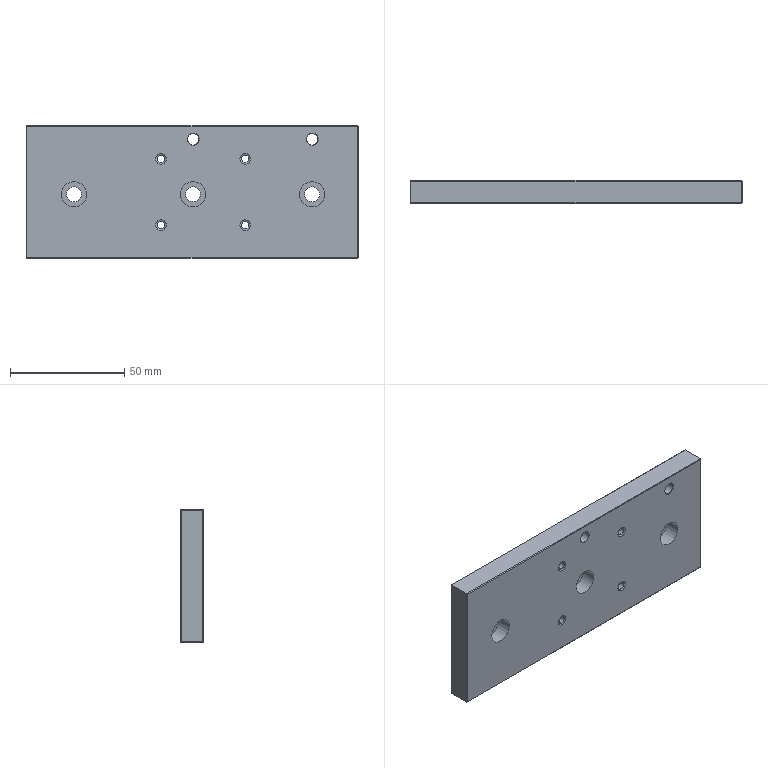Part | NX | 1 solid | 73 faces | box 145 x 10 x 58 mm | volume 81027 mm3 | cylinder 32 | plane 21 | cone 20 | commonest cylinder face diameters 2.5 x8 3.3 x8 6.5 x6 11 x6 5 x4